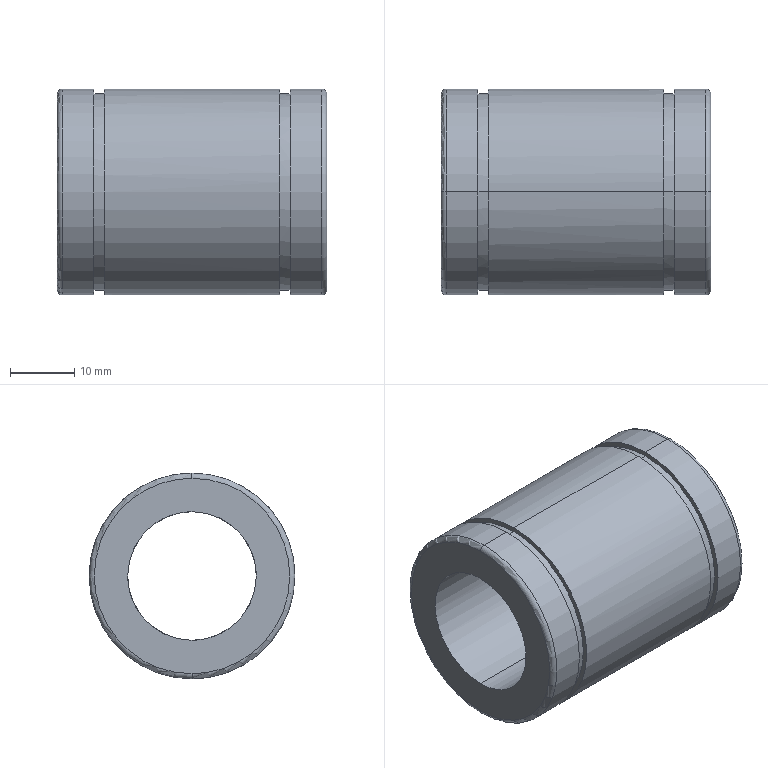Part | STEP file | _LMU-N20 | 1 solid | 22 faces | box 42 x 32 x 32 mm | volume 20321 mm3 | cylinder 12 | plane 6 | torus 4 | commonest cylinder face diameters 32 x6 30.5 x4 20 x2
STEP:
#1=CARTESIAN_POINT('',(0.,0.,-15.2));
#2=VERTEX_POINT('',#1);
#3=CARTESIAN_POINT('',(0.,15.2,0.));
#4=VERTEX_POINT('',#3);
#5=CARTESIAN_POINT('',(0.,0.,-15.2));
#6=CARTESIAN_POINT('',(0.,1.337,-15.2));
#7=CARTESIAN_POINT('',(0.,2.673,-15.053));
#8=CARTESIAN_POINT('',(0.,3.989,-14.759));
#9=CARTESIAN_POINT('',(0.,6.715,-13.825));
#10=CARTESIAN_POINT('',(0.,9.154,-12.28));
#11=CARTESIAN_POINT('',(0.,10.344,-11.295));
#12=CARTESIAN_POINT('',(0.,12.451,-9.049));
#13=CARTESIAN_POINT('',(0.,13.937,-6.351));
#14=CARTESIAN_POINT('',(0.,14.506,-4.915));
#15=CARTESIAN_POINT('',(0.,14.984,-3.05));
#16=CARTESIAN_POINT('',(0.,15.164,-1.147));
#17=CARTESIAN_POINT('',(0.,15.188,-0.7649));
#18=CARTESIAN_POINT('',(0.,15.2,-0.3824));
#19=CARTESIAN_POINT('',(0.,15.2,0.));
#20=B_SPLINE_CURVE_WITH_KNOTS('',5,(#5,#6,#7,#8,#9,#10,#11,#12,#13,#14,#15,#16,#17,#18,#19),.UNSPECIFIED.,.F.,.U.,(6,3,3,3,6),(33.766,43.217,54.022,64.826,67.53),.UNSPECIFIED.);
#21=EDGE_CURVE('',#2,#4,#20,.T.);
#22=ORIENTED_EDGE('',*,*,#21,.F.);
#23=CARTESIAN_POINT('',(0.,-15.2,0.));
#24=VERTEX_POINT('',#23);
#25=CARTESIAN_POINT('',(0.,-15.2,0.));
#26=CARTESIAN_POINT('',(0.,-15.2,-1.528));
#27=CARTESIAN_POINT('',(0.,-15.008,-3.056));
#28=CARTESIAN_POINT('',(0.,-14.624,-4.552));
#29=CARTESIAN_POINT('',(0.,-13.488,-7.415));
#30=CARTESIAN_POINT('',(0.,-11.68,-9.908));
#31=CARTESIAN_POINT('',(0.,-10.623,-11.034));
#32=CARTESIAN_POINT('',(0.,-8.248,-12.995));
#33=CARTESIAN_POINT('',(0.,-5.462,-14.309));
#34=CARTESIAN_POINT('',(0.,-3.994,-14.786));
#35=CARTESIAN_POINT('',(0.,-2.291,-15.11));
#36=CARTESIAN_POINT('',(0.,-0.5738,-15.191));
#37=CARTESIAN_POINT('',(0.,-0.3826,-15.197));
#38=CARTESIAN_POINT('',(0.,-0.1913,-15.2));
#39=CARTESIAN_POINT('',(0.,0.,-15.2));
#40=B_SPLINE_CURVE_WITH_KNOTS('',5,(#25,#26,#27,#28,#29,#30,#31,#32,#33,#34,#35,#36,#37,#38,#39),.UNSPECIFIED.,.F.,.U.,(6,3,3,3,6),(0.,10.804,21.609,32.413,33.766),.UNSPECIFIED.);
#41=EDGE_CURVE('',#24,#2,#40,.T.);
#42=ORIENTED_EDGE('',*,*,#41,.F.);
#43=CARTESIAN_POINT('',(0.,0.,15.2));
#44=VERTEX_POINT('',#43);
#45=CARTESIAN_POINT('',(0.,0.,15.2));
#46=CARTESIAN_POINT('',(0.,-1.337,15.2));
#47=CARTESIAN_POINT('',(0.,-2.673,15.053));
#48=CARTESIAN_POINT('',(0.,-3.989,14.759));
#49=CARTESIAN_POINT('',(0.,-6.715,13.825));
#50=CARTESIAN_POINT('',(0.,-9.154,12.28));
#51=CARTESIAN_POINT('',(0.,-10.344,11.295));
#52=CARTESIAN_POINT('',(0.,-12.451,9.049));
#53=CARTESIAN_POINT('',(0.,-13.937,6.351));
#54=CARTESIAN_POINT('',(0.,-14.506,4.915));
#55=CARTESIAN_POINT('',(0.,-14.984,3.05));
#56=CARTESIAN_POINT('',(0.,-15.164,1.147));
#57=CARTESIAN_POINT('',(0.,-15.188,0.7649));
#58=CARTESIAN_POINT('',(0.,-15.2,0.3824));
#59=CARTESIAN_POINT('',(0.,-15.2,0.));
#60=B_SPLINE_CURVE_WITH_KNOTS('',5,(#45,#46,#47,#48,#49,#50,#51,#52,#53,#54,#55,#56,#57,#58,#59),.UNSPECIFIED.,.F.,.U.,(6,3,3,3,6),(33.766,43.217,54.022,64.826,67.53),.UNSPECIFIED.);
#61=EDGE_CURVE('',#44,#24,#60,.T.);
#62=ORIENTED_EDGE('',*,*,#61,.F.);
#63=CARTESIAN_POINT('',(0.,15.2,0.));
#64=CARTESIAN_POINT('',(0.,15.2,1.528));
#65=CARTESIAN_POINT('',(0.,15.008,3.056));
#66=CARTESIAN_POINT('',(0.,14.624,4.552));
#67=CARTESIAN_POINT('',(0.,13.488,7.415));
#68=CARTESIAN_POINT('',(0.,11.68,9.908));
#69=CARTESIAN_POINT('',(0.,10.623,11.034));
#70=CARTESIAN_POINT('',(0.,8.248,12.995));
#71=CARTESIAN_POINT('',(0.,5.462,14.309));
#72=CARTESIAN_POINT('',(0.,3.994,14.786));
#73=CARTESIAN_POINT('',(0.,2.291,15.11));
#74=CARTESIAN_POINT('',(0.,0.5738,15.191));
#75=CARTESIAN_POINT('',(0.,0.3826,15.197));
#76=CARTESIAN_POINT('',(0.,0.1913,15.2));
#77=CARTESIAN_POINT('',(0.,0.,15.2));
#78=B_SPLINE_CURVE_WITH_KNOTS('',5,(#63,#64,#65,#66,#67,#68,#69,#70,#71,#72,#73,#74,#75,#76,#77),.UNSPECIFIED.,.F.,.U.,(6,3,3,3,6),(0.,10.804,21.609,32.413,33.766),.UNSPECIFIED.);
#79=EDGE_CURVE('',#4,#44,#78,.T.);
#80=ORIENTED_EDGE('',*,*,#79,.F.);
#81=EDGE_LOOP('',(#22,#42,#62,#80));
#82=FACE_OUTER_BOUND('',#81,.T.);
#83=CARTESIAN_POINT('',(0.,10.,0.));
#84=VERTEX_POINT('',#83);
#85=CARTESIAN_POINT('',(0.,0.,10.));
#86=VERTEX_POINT('',#85);
#87=CARTESIAN_POINT('',(0.,10.,0.));
#88=CARTESIAN_POINT('',(0.,10.,0.9295));
#89=CARTESIAN_POINT('',(0.,9.892,1.859));
#90=CARTESIAN_POINT('',(0.,9.676,2.772));
#91=CARTESIAN_POINT('',(0.,9.036,4.53));
#92=CARTESIAN_POINT('',(0.,8.01,6.095));
#93=CARTESIAN_POINT('',(0.,7.407,6.815));
#94=CARTESIAN_POINT('',(0.,6.047,8.1));
#95=CARTESIAN_POINT('',(0.,4.428,9.039));
#96=CARTESIAN_POINT('',(0.,3.567,9.412));
#97=CARTESIAN_POINT('',(0.,2.331,9.784));
#98=CARTESIAN_POINT('',(0.,1.058,9.953));
#99=CARTESIAN_POINT('',(0.,0.7061,9.984));
#100=CARTESIAN_POINT('',(0.,0.353,10.));
#101=CARTESIAN_POINT('',(0.,0.,10.));
#102=B_SPLINE_CURVE_WITH_KNOTS('',5,(#87,#88,#89,#90,#91,#92,#93,#94,#95,#96,#97,#98,#99,#100,#101),.UNSPECIFIED.,.F.,.U.,(6,3,3,3,6),(0.,6.573,13.145,19.718,22.214),.UNSPECIFIED.);
#103=EDGE_CURVE('',#84,#86,#102,.T.);
#104=ORIENTED_EDGE('',*,*,#103,.T.);
#105=CARTESIAN_POINT('',(0.,-10.,0.));
#106=VERTEX_POINT('',#105);
#107=CARTESIAN_POINT('',(0.,0.,10.));
#108=CARTESIAN_POINT('',(0.,-0.5765,10.));
#109=CARTESIAN_POINT('',(0.,-1.153,9.958));
#110=CARTESIAN_POINT('',(0.,-1.725,9.875));
#111=CARTESIAN_POINT('',(0.,-3.2,9.551));
#112=CARTESIAN_POINT('',(0.,-4.594,8.955));
#113=CARTESIAN_POINT('',(0.,-5.408,8.489));
#114=CARTESIAN_POINT('',(0.,-6.912,7.375));
#115=CARTESIAN_POINT('',(0.,-8.121,5.946));
#116=CARTESIAN_POINT('',(0.,-8.639,5.165));
#117=CARTESIAN_POINT('',(0.,-9.383,3.696));
#118=CARTESIAN_POINT('',(0.,-9.813,2.111));
#119=CARTESIAN_POINT('',(0.,-9.938,1.412));
#120=CARTESIAN_POINT('',(0.,-10.,0.7061));
#121=CARTESIAN_POINT('',(0.,-10.,0.));
#122=B_SPLINE_CURVE_WITH_KNOTS('',5,(#107,#108,#109,#110,#111,#112,#113,#114,#115,#116,#117,#118,#119,#120,#121),.UNSPECIFIED.,.F.,.U.,(6,3,3,3,6),(22.214,26.29,32.863,39.436,44.428),.UNSPECIFIED.);
#123=EDGE_CURVE('',#86,#106,#122,.T.);
#124=ORIENTED_EDGE('',*,*,#123,.T.);
#125=CARTESIAN_POINT('',(0.,0.,-10.));
#126=VERTEX_POINT('',#125);
#127=CARTESIAN_POINT('',(0.,-10.,0.));
#128=CARTESIAN_POINT('',(0.,-10.,-0.9295));
#129=CARTESIAN_POINT('',(0.,-9.892,-1.859));
#130=CARTESIAN_POINT('',(0.,-9.676,-2.772));
#131=CARTESIAN_POINT('',(0.,-9.036,-4.53));
#132=CARTESIAN_POINT('',(0.,-8.01,-6.095));
#133=CARTESIAN_POINT('',(0.,-7.407,-6.815));
#134=CARTESIAN_POINT('',(0.,-6.047,-8.1));
#135=CARTESIAN_POINT('',(0.,-4.428,-9.039));
#136=CARTESIAN_POINT('',(0.,-3.567,-9.412));
#137=CARTESIAN_POINT('',(0.,-2.331,-9.784));
#138=CARTESIAN_POINT('',(0.,-1.058,-9.953));
#139=CARTESIAN_POINT('',(0.,-0.7061,-9.984));
#140=CARTESIAN_POINT('',(0.,-0.353,-10.));
#141=CARTESIAN_POINT('',(0.,0.,-10.));
#142=B_SPLINE_CURVE_WITH_KNOTS('',5,(#127,#128,#129,#130,#131,#132,#133,#134,#135,#136,#137,#138,#139,#140,#141),.UNSPECIFIED.,.F.,.U.,(6,3,3,3,6),(0.,6.573,13.145,19.718,22.214),.UNSPECIFIED.);
#143=EDGE_CURVE('',#106,#126,#142,.T.);
#144=ORIENTED_EDGE('',*,*,#143,.T.);
#145=CARTESIAN_POINT('',(0.,0.,-10.));
#146=CARTESIAN_POINT('',(0.,0.5765,-10.));
#147=CARTESIAN_POINT('',(0.,1.153,-9.958));
#148=CARTESIAN_POINT('',(0.,1.725,-9.875));
#149=CARTESIAN_POINT('',(0.,3.2,-9.551));
#150=CARTESIAN_POINT('',(0.,4.594,-8.955));
#151=CARTESIAN_POINT('',(0.,5.408,-8.489));
#152=CARTESIAN_POINT('',(0.,6.912,-7.375));
#153=CARTESIAN_POINT('',(0.,8.121,-5.946));
#154=CARTESIAN_POINT('',(0.,8.639,-5.165));
#155=CARTESIAN_POINT('',(0.,9.383,-3.696));
#156=CARTESIAN_POINT('',(0.,9.813,-2.111));
#157=CARTESIAN_POINT('',(0.,9.938,-1.412));
#158=CARTESIAN_POINT('',(0.,10.,-0.7061));
#159=CARTESIAN_POINT('',(0.,10.,0.));
#160=B_SPLINE_CURVE_WITH_KNOTS('',5,(#145,#146,#147,#148,#149,#150,#151,#152,#153,#154,#155,#156,#157,#158,#159),.UNSPECIFIED.,.F.,.U.,(6,3,3,3,6),(22.214,26.29,32.863,39.436,44.428),.UNSPECIFIED.);
#161=EDGE_CURVE('',#126,#84,#160,.T.);
#162=ORIENTED_EDGE('',*,*,#161,.T.);
#163=EDGE_LOOP('',(#104,#124,#144,#162));
#164=FACE_BOUND('',#163,.T.);
#165=CARTESIAN_POINT('',(0.,15.2,0.));
#166=DIRECTION('',(-1.,0.,0.));
#167=DIRECTION('',(0.,0.,1.));
#168=AXIS2_PLACEMENT_3D('',#165,#166,#167);
#169=PLANE('',#168);
#170=ADVANCED_FACE('',(#82,#164),#169,.T.);
#171=CARTESIAN_POINT('',(0.8,0.,16.));
#172=VERTEX_POINT('',#171);
#173=CARTESIAN_POINT('',(0.8,0.,15.2));
#174=DIRECTION('',(0.,1.,0.));
#175=AXIS2_PLACEMENT_3D('',#173,#174,$);
#176=CIRCLE('',#175,0.8);
#177=EDGE_CURVE('',#44,#172,#176,.T.);
#178=ORIENTED_EDGE('',*,*,#177,.T.);
#179=CARTESIAN_POINT('',(0.8,16.,0.));
#180=VERTEX_POINT('',#179);
#181=CARTESIAN_POINT('',(0.8,0.,0.));
#182=DIRECTION('',(1.,0.,0.));
#183=AXIS2_PLACEMENT_3D('',#181,#182,$);
#184=CIRCLE('',#183,16.);
#185=EDGE_CURVE('',#180,#172,#184,.T.);
#186=ORIENTED_EDGE('',*,*,#185,.F.);
#187=CARTESIAN_POINT('',(0.8,0.,-16.));
#188=VERTEX_POINT('',#187);
#189=CARTESIAN_POINT('',(0.8,0.,0.));
#190=DIRECTION('',(1.,0.,0.));
#191=AXIS2_PLACEMENT_3D('',#189,#190,$);
#192=CIRCLE('',#191,16.);
#193=EDGE_CURVE('',#188,#180,#192,.T.);
#194=ORIENTED_EDGE('',*,*,#193,.F.);
#195=CARTESIAN_POINT('',(0.8,0.,-15.2));
#196=DIRECTION('',(0.,-1.,0.));
#197=AXIS2_PLACEMENT_3D('',#195,#196,$);
#198=CIRCLE('',#197,0.8);
#199=EDGE_CURVE('',#188,#2,#198,.F.);
#200=ORIENTED_EDGE('',*,*,#199,.T.);
#201=ORIENTED_EDGE('',*,*,#21,.T.);
#202=ORIENTED_EDGE('',*,*,#79,.T.);
#203=EDGE_LOOP('',(#178,#186,#194,#200,#201,#202));
#204=FACE_OUTER_BOUND('',#203,.T.);
#205=CARTESIAN_POINT('',(0.8,0.,0.));
#206=DIRECTION('',(1.,0.,0.));
#207=DIRECTION('',(0.,0.,-1.));
#208=AXIS2_PLACEMENT_3D('',#205,#206,#207);
#209=TOROIDAL_SURFACE('',#208,15.2,0.8);
#210=ADVANCED_FACE('',(#204),#209,.T.);
#211=ORIENTED_EDGE('',*,*,#199,.F.);
#212=CARTESIAN_POINT('',(0.8,-16.,0.));
#213=VERTEX_POINT('',#212);
#214=CARTESIAN_POINT('',(0.8,0.,0.));
#215=DIRECTION('',(1.,0.,0.));
#216=AXIS2_PLACEMENT_3D('',#214,#215,$);
#217=CIRCLE('',#216,16.);
#218=EDGE_CURVE('',#213,#188,#217,.T.);
#219=ORIENTED_EDGE('',*,*,#218,.F.);
#220=CARTESIAN_POINT('',(0.8,0.,0.));
#221=DIRECTION('',(1.,0.,0.));
#222=AXIS2_PLACEMENT_3D('',#220,#221,$);
#223=CIRCLE('',#222,16.);
#224=EDGE_CURVE('',#172,#213,#223,.T.);
#225=ORIENTED_EDGE('',*,*,#224,.F.);
#226=ORIENTED_EDGE('',*,*,#177,.F.);
#227=ORIENTED_EDGE('',*,*,#61,.T.);
#228=ORIENTED_EDGE('',*,*,#41,.T.);
#229=EDGE_LOOP('',(#211,#219,#225,#226,#227,#228));
#230=FACE_OUTER_BOUND('',#229,.T.);
#231=CARTESIAN_POINT('',(0.8,0.,0.));
#232=DIRECTION('',(1.,0.,0.));
#233=DIRECTION('',(0.,0.,1.));
#234=AXIS2_PLACEMENT_3D('',#231,#232,#233);
#235=TOROIDAL_SURFACE('',#234,15.2,0.8);
#236=ADVANCED_FACE('',(#230),#235,.T.);
#237=CARTESIAN_POINT('',(42.,0.,-10.));
#238=VERTEX_POINT('',#237);
#239=CARTESIAN_POINT('',(42.,10.,0.));
#240=VERTEX_POINT('',#239);
#241=CARTESIAN_POINT('',(42.,0.,0.));
#242=DIRECTION('',(-1.,0.,0.));
#243=AXIS2_PLACEMENT_3D('',#241,#242,$);
#244=CIRCLE('',#243,10.);
#245=EDGE_CURVE('',#238,#240,#244,.F.);
#246=ORIENTED_EDGE('',*,*,#245,.T.);
#247=CARTESIAN_POINT('',(42.,0.,10.));
#248=VERTEX_POINT('',#247);
#249=CARTESIAN_POINT('',(42.,0.,0.));
#250=DIRECTION('',(-1.,0.,0.));
#251=AXIS2_PLACEMENT_3D('',#249,#250,$);
#252=CIRCLE('',#251,10.);
#253=EDGE_CURVE('',#240,#248,#252,.F.);
#254=ORIENTED_EDGE('',*,*,#253,.T.);
#255=CARTESIAN_POINT('',(42.,0.,10.));
#256=DIRECTION('',(-1.,0.,0.));
#257=VECTOR('',#256,1.);
#258=LINE('',#255,#257);
#259=EDGE_CURVE('',#248,#86,#258,.T.);
#260=ORIENTED_EDGE('',*,*,#259,.T.);
#261=ORIENTED_EDGE('',*,*,#103,.F.);
#262=ORIENTED_EDGE('',*,*,#161,.F.);
#263=CARTESIAN_POINT('',(42.,0.,-10.));
#264=DIRECTION('',(-1.,0.,0.));
#265=VECTOR('',#264,1.);
#266=LINE('',#263,#265);
#267=EDGE_CURVE('',#126,#238,#266,.F.);
#268=ORIENTED_EDGE('',*,*,#267,.T.);
#269=EDGE_LOOP('',(#246,#254,#260,#261,#262,#268));
#270=FACE_OUTER_BOUND('',#269,.T.);
#271=CARTESIAN_POINT('',(42.,0.,0.));
#272=DIRECTION('',(-1.,0.,0.));
#273=DIRECTION('',(0.,0.,1.));
#274=AXIS2_PLACEMENT_3D('',#271,#272,#273);
#275=CYLINDRICAL_SURFACE('',#274,10.);
#276=ADVANCED_FACE('',(#270),#275,.F.);
#277=CARTESIAN_POINT('',(42.,-10.,0.));
#278=VERTEX_POINT('',#277);
#279=CARTESIAN_POINT('',(42.,0.,0.));
#280=DIRECTION('',(-1.,0.,0.));
#281=AXIS2_PLACEMENT_3D('',#279,#280,$);
#282=CIRCLE('',#281,10.);
#283=EDGE_CURVE('',#248,#278,#282,.F.);
#284=ORIENTED_EDGE('',*,*,#283,.T.);
#285=CARTESIAN_POINT('',(42.,0.,0.));
#286=DIRECTION('',(-1.,0.,0.));
#287=AXIS2_PLACEMENT_3D('',#285,#286,$);
#288=CIRCLE('',#287,10.);
#289=EDGE_CURVE('',#278,#238,#288,.F.);
#290=ORIENTED_EDGE('',*,*,#289,.T.);
#291=ORIENTED_EDGE('',*,*,#267,.F.);
#292=ORIENTED_EDGE('',*,*,#143,.F.);
#293=ORIENTED_EDGE('',*,*,#123,.F.);
#294=ORIENTED_EDGE('',*,*,#259,.F.);
#295=EDGE_LOOP('',(#284,#290,#291,#292,#293,#294));
#296=FACE_OUTER_BOUND('',#295,.T.);
#297=CARTESIAN_POINT('',(42.,0.,0.));
#298=DIRECTION('',(-1.,0.,0.));
#299=DIRECTION('',(0.,0.,-1.));
#300=AXIS2_PLACEMENT_3D('',#297,#298,#299);
#301=CYLINDRICAL_SURFACE('',#300,10.);
#302=ADVANCED_FACE('',(#296),#301,.F.);
#303=CARTESIAN_POINT('',(5.75,0.,16.));
#304=VERTEX_POINT('',#303);
#305=CARTESIAN_POINT('',(42.,0.,16.));
#306=DIRECTION('',(-1.,0.,0.));
#307=VECTOR('',#306,1.);
#308=LINE('',#305,#307);
#309=EDGE_CURVE('',#304,#172,#308,.T.);
#310=ORIENTED_EDGE('',*,*,#309,.F.);
#311=CARTESIAN_POINT('',(5.75,16.,0.));
#312=VERTEX_POINT('',#311);
#313=CARTESIAN_POINT('',(5.75,0.,0.));
#314=DIRECTION('',(-1.,0.,0.));
#315=AXIS2_PLACEMENT_3D('',#313,#314,$);
#316=CIRCLE('',#315,16.);
#317=EDGE_CURVE('',#312,#304,#316,.F.);
#318=ORIENTED_EDGE('',*,*,#317,.F.);
#319=CARTESIAN_POINT('',(5.75,0.,-16.));
#320=VERTEX_POINT('',#319);
#321=CARTESIAN_POINT('',(5.75,0.,0.));
#322=DIRECTION('',(-1.,0.,0.));
#323=AXIS2_PLACEMENT_3D('',#321,#322,$);
#324=CIRCLE('',#323,16.);
#325=EDGE_CURVE('',#320,#312,#324,.F.);
#326=ORIENTED_EDGE('',*,*,#325,.F.);
#327=CARTESIAN_POINT('',(42.,0.,-16.));
#328=DIRECTION('',(-1.,0.,0.));
#329=VECTOR('',#328,1.);
#330=LINE('',#327,#329);
#331=EDGE_CURVE('',#188,#320,#330,.F.);
#332=ORIENTED_EDGE('',*,*,#331,.F.);
#333=ORIENTED_EDGE('',*,*,#193,.T.);
#334=ORIENTED_EDGE('',*,*,#185,.T.);
#335=EDGE_LOOP('',(#310,#318,#326,#332,#333,#334));
#336=FACE_OUTER_BOUND('',#335,.T.);
#337=CARTESIAN_POINT('',(42.,0.,0.));
#338=DIRECTION('',(-1.,0.,0.));
#339=DIRECTION('',(0.,0.,1.));
#340=AXIS2_PLACEMENT_3D('',#337,#338,#339);
#341=CYLINDRICAL_SURFACE('',#340,16.);
#342=ADVANCED_FACE('',(#336),#341,.T.);
#343=ORIENTED_EDGE('',*,*,#331,.T.);
#344=CARTESIAN_POINT('',(5.75,-16.,0.));
#345=VERTEX_POINT('',#344);
#346=CARTESIAN_POINT('',(5.75,0.,0.));
#347=DIRECTION('',(-1.,0.,0.));
#348=AXIS2_PLACEMENT_3D('',#346,#347,$);
#349=CIRCLE('',#348,16.);
#350=EDGE_CURVE('',#345,#320,#349,.F.);
#351=ORIENTED_EDGE('',*,*,#350,.F.);
#352=CARTESIAN_POINT('',(5.75,0.,0.));
#353=DIRECTION('',(-1.,0.,0.));
#354=AXIS2_PLACEMENT_3D('',#352,#353,$);
#355=CIRCLE('',#354,16.);
#356=EDGE_CURVE('',#304,#345,#355,.F.);
#357=ORIENTED_EDGE('',*,*,#356,.F.);
#358=ORIENTED_EDGE('',*,*,#309,.T.);
#359=ORIENTED_EDGE('',*,*,#224,.T.);
#360=ORIENTED_EDGE('',*,*,#218,.T.);
#361=EDGE_LOOP('',(#343,#351,#357,#358,#359,#360));
#362=FACE_OUTER_BOUND('',#361,.T.);
#363=CARTESIAN_POINT('',(42.,0.,0.));
#364=DIRECTION('',(-1.,0.,0.));
#365=DIRECTION('',(0.,0.,-1.));
#366=AXIS2_PLACEMENT_3D('',#363,#364,#365);
#367=CYLINDRICAL_SURFACE('',#366,16.);
#368=ADVANCED_FACE('',(#362),#367,.T.);
#369=CARTESIAN_POINT('',(42.,15.2,0.));
#370=VERTEX_POINT('',#369);
#371=CARTESIAN_POINT('',(42.,0.,15.2));
#372=VERTEX_POINT('',#371);
#373=CARTESIAN_POINT('',(42.,0.,0.));
#374=DIRECTION('',(1.,0.,0.));
#375=AXIS2_PLACEMENT_3D('',#373,#374,$);
#376=CIRCLE('',#375,15.2);
#377=EDGE_CURVE('',#370,#372,#376,.T.);
#378=ORIENTED_EDGE('',*,*,#377,.T.);
#379=CARTESIAN_POINT('',(42.,-15.2,0.));
#380=VERTEX_POINT('',#379);
#381=CARTESIAN_POINT('',(42.,0.,0.));
#382=DIRECTION('',(1.,0.,0.));
#383=AXIS2_PLACEMENT_3D('',#381,#382,$);
#384=CIRCLE('',#383,15.2);
#385=EDGE_CURVE('',#372,#380,#384,.T.);
#386=ORIENTED_EDGE('',*,*,#385,.T.);
#387=CARTESIAN_POINT('',(42.,0.,-15.2));
#388=VERTEX_POINT('',#387);
#389=CARTESIAN_POINT('',(42.,0.,0.));
#390=DIRECTION('',(1.,0.,0.));
#391=AXIS2_PLACEMENT_3D('',#389,#390,$);
#392=CIRCLE('',#391,15.2);
#393=EDGE_CURVE('',#380,#388,#392,.T.);
#394=ORIENTED_EDGE('',*,*,#393,.T.);
#395=CARTESIAN_POINT('',(42.,0.,0.));
#396=DIRECTION('',(1.,0.,0.));
#397=AXIS2_PLACEMENT_3D('',#395,#396,$);
#398=CIRCLE('',#397,15.2);
#399=EDGE_CURVE('',#388,#370,#398,.T.);
#400=ORIENTED_EDGE('',*,*,#399,.T.);
#401=EDGE_LOOP('',(#378,#386,#394,#400));
#402=FACE_OUTER_BOUND('',#401,.T.);
#403=ORIENTED_EDGE('',*,*,#245,.F.);
#404=ORIENTED_EDGE('',*,*,#289,.F.);
#405=ORIENTED_EDGE('',*,*,#283,.F.);
#406=ORIENTED_EDGE('',*,*,#253,.F.);
#407=EDGE_LOOP('',(#403,#404,#405,#406));
#408=FACE_BOUND('',#407,.T.);
#409=CARTESIAN_POINT('',(42.,10.,0.));
#410=DIRECTION('',(1.,0.,0.));
#411=DIRECTION('',(0.,0.,-1.));
#412=AXIS2_PLACEMENT_3D('',#409,#410,#411);
#413=PLANE('',#412);
#414=ADVANCED_FACE('',(#402,#408),#413,.T.);
#415=ORIENTED_EDGE('',*,*,#317,.T.);
#416=ORIENTED_EDGE('',*,*,#356,.T.);
#417=ORIENTED_EDGE('',*,*,#350,.T.);
#418=ORIENTED_EDGE('',*,*,#325,.T.);
#419=EDGE_LOOP('',(#415,#416,#417,#418));
#420=FACE_OUTER_BOUND('',#419,.T.);
#421=CARTESIAN_POINT('',(5.75,0.,-15.25));
#422=VERTEX_POINT('',#421);
#423=CARTESIAN_POINT('',(5.75,15.25,0.));
#424=VERTEX_POINT('',#423);
#425=CARTESIAN_POINT('',(5.75,0.,0.));
#426=DIRECTION('',(1.,0.,0.));
#427=AXIS2_PLACEMENT_3D('',#425,#426,$);
#428=CIRCLE('',#427,15.25);
#429=EDGE_CURVE('',#422,#424,#428,.T.);
#430=ORIENTED_EDGE('',*,*,#429,.F.);
#431=CARTESIAN_POINT('',(5.75,-15.25,0.));
#432=VERTEX_POINT('',#431);
#433=CARTESIAN_POINT('',(5.75,0.,0.));
#434=DIRECTION('',(1.,0.,0.));
#435=AXIS2_PLACEMENT_3D('',#433,#434,$);
#436=CIRCLE('',#435,15.25);
#437=EDGE_CURVE('',#432,#422,#436,.T.);
#438=ORIENTED_EDGE('',*,*,#437,.F.);
#439=CARTESIAN_POINT('',(5.75,0.,15.25));
#440=VERTEX_POINT('',#439);
#441=CARTESIAN_POINT('',(5.75,0.,0.));
#442=DIRECTION('',(1.,0.,0.));
#443=AXIS2_PLACEMENT_3D('',#441,#442,$);
#444=CIRCLE('',#443,15.25);
#445=EDGE_CURVE('',#440,#432,#444,.T.);
#446=ORIENTED_EDGE('',*,*,#445,.F.);
#447=CARTESIAN_POINT('',(5.75,0.,0.));
#448=DIRECTION('',(1.,0.,0.));
#449=AXIS2_PLACEMENT_3D('',#447,#448,$);
#450=CIRCLE('',#449,15.25);
#451=EDGE_CURVE('',#424,#440,#450,.T.);
#452=ORIENTED_EDGE('',*,*,#451,.F.);
#453=EDGE_LOOP('',(#430,#438,#446,#452));
#454=FACE_BOUND('',#453,.T.);
#455=CARTESIAN_POINT('',(5.75,15.25,0.));
#456=DIRECTION('',(1.,0.,0.));
#457=DIRECTION('',(0.,0.,-1.));
#458=AXIS2_PLACEMENT_3D('',#455,#456,#457);
#459=PLANE('',#458);
#460=ADVANCED_FACE('',(#420,#454),#459,.T.);
#461=CARTESIAN_POINT('',(41.2,0.,16.));
#462=VERTEX_POINT('',#461);
#463=CARTESIAN_POINT('',(41.2,0.,15.2));
#464=DIRECTION('',(0.,1.,0.));
#465=AXIS2_PLACEMENT_3D('',#463,#464,$);
#466=CIRCLE('',#465,0.8);
#467=EDGE_CURVE('',#462,#372,#466,.T.);
#468=ORIENTED_EDGE('',*,*,#467,.T.);
#469=ORIENTED_EDGE('',*,*,#377,.F.);
#470=ORIENTED_EDGE('',*,*,#399,.F.);
#471=CARTESIAN_POINT('',(41.2,0.,-16.));
#472=VERTEX_POINT('',#471);
#473=CARTESIAN_POINT('',(41.2,0.,-15.2));
#474=DIRECTION('',(0.,-1.,0.));
#475=AXIS2_PLACEMENT_3D('',#473,#474,$);
#476=CIRCLE('',#475,0.8);
#477=EDGE_CURVE('',#388,#472,#476,.F.);
#478=ORIENTED_EDGE('',*,*,#477,.T.);
#479=CARTESIAN_POINT('',(41.2,16.,0.));
#480=VERTEX_POINT('',#479);
#481=CARTESIAN_POINT('',(41.2,0.,0.));
#482=DIRECTION('',(1.,0.,0.));
#483=AXIS2_PLACEMENT_3D('',#481,#482,$);
#484=CIRCLE('',#483,16.);
#485=EDGE_CURVE('',#472,#480,#484,.T.);
#486=ORIENTED_EDGE('',*,*,#485,.T.);
#487=CARTESIAN_POINT('',(41.2,0.,0.));
#488=DIRECTION('',(1.,0.,0.));
#489=AXIS2_PLACEMENT_3D('',#487,#488,$);
#490=CIRCLE('',#489,16.);
#491=EDGE_CURVE('',#480,#462,#490,.T.);
#492=ORIENTED_EDGE('',*,*,#491,.T.);
#493=EDGE_LOOP('',(#468,#469,#470,#478,#486,#492));
#494=FACE_OUTER_BOUND('',#493,.T.);
#495=CARTESIAN_POINT('',(41.2,0.,0.));
#496=DIRECTION('',(1.,0.,0.));
#497=DIRECTION('',(0.,0.,-1.));
#498=AXIS2_PLACEMENT_3D('',#495,#496,#497);
#499=TOROIDAL_SURFACE('',#498,15.2,0.8);
#500=ADVANCED_FACE('',(#494),#499,.T.);
#501=ORIENTED_EDGE('',*,*,#477,.F.);
#502=ORIENTED_EDGE('',*,*,#393,.F.);
#503=ORIENTED_EDGE('',*,*,#385,.F.);
#504=ORIENTED_EDGE('',*,*,#467,.F.);
#505=CARTESIAN_POINT('',(41.2,-16.,0.));
#506=VERTEX_POINT('',#505);
#507=CARTESIAN_POINT('',(41.2,0.,0.));
#508=DIRECTION('',(1.,0.,0.));
#509=AXIS2_PLACEMENT_3D('',#507,#508,$);
#510=CIRCLE('',#509,16.);
#511=EDGE_CURVE('',#462,#506,#510,.T.);
#512=ORIENTED_EDGE('',*,*,#511,.T.);
#513=CARTESIAN_POINT('',(41.2,0.,0.));
#514=DIRECTION('',(1.,0.,0.));
#515=AXIS2_PLACEMENT_3D('',#513,#514,$);
#516=CIRCLE('',#515,16.);
#517=EDGE_CURVE('',#506,#472,#516,.T.);
#518=ORIENTED_EDGE('',*,*,#517,.T.);
#519=EDGE_LOOP('',(#501,#502,#503,#504,#512,#518));
#520=FACE_OUTER_BOUND('',#519,.T.);
#521=CARTESIAN_POINT('',(41.2,0.,0.));
#522=DIRECTION('',(1.,0.,0.));
#523=DIRECTION('',(0.,0.,1.));
#524=AXIS2_PLACEMENT_3D('',#521,#522,#523);
#525=TOROIDAL_SURFACE('',#524,15.2,0.8);
#526=ADVANCED_FACE('',(#520),#525,.T.);
#527=CARTESIAN_POINT('',(7.35,0.,15.25));
#528=VERTEX_POINT('',#527);
#529=CARTESIAN_POINT('',(42.,0.,15.25));
#530=DIRECTION('',(-1.,0.,0.));
#531=VECTOR('',#530,1.);
#532=LINE('',#529,#531);
#533=EDGE_CURVE('',#528,#440,#532,.T.);
#534=ORIENTED_EDGE('',*,*,#533,.F.);
#535=CARTESIAN_POINT('',(7.35,15.25,0.));
#536=VERTEX_POINT('',#535);
#537=CARTESIAN_POINT('',(7.35,15.25,0.));
#538=CARTESIAN_POINT('',(7.35,15.25,4.791));
#539=CARTESIAN_POINT('',(7.35,13.374,9.586));
#540=CARTESIAN_POINT('',(7.35,9.586,13.374));
#541=CARTESIAN_POINT('',(7.35,4.791,15.25));
#542=CARTESIAN_POINT('',(7.35,0.,15.25));
#543=B_SPLINE_CURVE_WITH_KNOTS('',5,(#537,#538,#539,#540,#541,#542),.UNSPECIFIED.,.F.,.U.,(6,6),(-11.977,11.977),.UNSPECIFIED.);
#544=EDGE_CURVE('',#536,#528,#543,.T.);
#545=ORIENTED_EDGE('',*,*,#544,.F.);
#546=CARTESIAN_POINT('',(7.35,0.,-15.25));
#547=VERTEX_POINT('',#546);
#548=CARTESIAN_POINT('',(7.35,0.,0.));
#549=DIRECTION('',(-1.,0.,0.));
#550=AXIS2_PLACEMENT_3D('',#548,#549,$);
#551=CIRCLE('',#550,15.25);
#552=EDGE_CURVE('',#547,#536,#551,.F.);
#553=ORIENTED_EDGE('',*,*,#552,.F.);
#554=CARTESIAN_POINT('',(42.,0.,-15.25));
#555=DIRECTION('',(-1.,0.,0.));
#556=VECTOR('',#555,1.);
#557=LINE('',#554,#556);
#558=EDGE_CURVE('',#422,#547,#557,.F.);
#559=ORIENTED_EDGE('',*,*,#558,.F.);
#560=ORIENTED_EDGE('',*,*,#429,.T.);
#561=ORIENTED_EDGE('',*,*,#451,.T.);
#562=EDGE_LOOP('',(#534,#545,#553,#559,#560,#561));
#563=FACE_OUTER_BOUND('',#562,.T.);
#564=CARTESIAN_POINT('',(42.,0.,0.));
#565=DIRECTION('',(-1.,0.,0.));
#566=DIRECTION('',(0.,0.,1.));
#567=AXIS2_PLACEMENT_3D('',#564,#565,#566);
#568=CYLINDRICAL_SURFACE('',#567,15.25);
#569=ADVANCED_FACE('',(#563),#568,.T.);
#570=ORIENTED_EDGE('',*,*,#558,.T.);
#571=CARTESIAN_POINT('',(7.35,-15.25,0.));
#572=VERTEX_POINT('',#571);
#573=CARTESIAN_POINT('',(7.35,0.,0.));
#574=DIRECTION('',(-1.,0.,0.));
#575=AXIS2_PLACEMENT_3D('',#573,#574,$);
#576=CIRCLE('',#575,15.25);
#577=EDGE_CURVE('',#572,#547,#576,.F.);
#578=ORIENTED_EDGE('',*,*,#577,.F.);
#579=CARTESIAN_POINT('',(7.35,0.,15.25));
#580=CARTESIAN_POINT('',(7.35,-4.791,15.25));
#581=CARTESIAN_POINT('',(7.35,-9.586,13.374));
#582=CARTESIAN_POINT('',(7.35,-13.374,9.586));
#583=CARTESIAN_POINT('',(7.35,-15.25,4.791));
#584=CARTESIAN_POINT('',(7.35,-15.25,0.));
#585=B_SPLINE_CURVE_WITH_KNOTS('',5,(#579,#580,#581,#582,#583,#584),.UNSPECIFIED.,.F.,.U.,(6,6),(-11.977,11.977),.UNSPECIFIED.);
#586=EDGE_CURVE('',#528,#572,#585,.T.);
#587=ORIENTED_EDGE('',*,*,#586,.F.);
#588=ORIENTED_EDGE('',*,*,#533,.T.);
#589=ORIENTED_EDGE('',*,*,#445,.T.);
#590=ORIENTED_EDGE('',*,*,#437,.T.);
#591=EDGE_LOOP('',(#570,#578,#587,#588,#589,#590));
#592=FACE_OUTER_BOUND('',#591,.T.);
#593=CARTESIAN_POINT('',(42.,0.,0.));
#594=DIRECTION('',(-1.,0.,0.));
#595=DIRECTION('',(0.,0.,-1.));
#596=AXIS2_PLACEMENT_3D('',#593,#594,#595);
#597=CYLINDRICAL_SURFACE('',#596,15.25);
#598=ADVANCED_FACE('',(#592),#597,.T.);
#599=CARTESIAN_POINT('',(36.25,0.,16.));
#600=VERTEX_POINT('',#599);
#601=CARTESIAN_POINT('',(42.,0.,16.));
#602=DIRECTION('',(-1.,0.,0.));
#603=VECTOR('',#602,1.);
#604=LINE('',#601,#603);
#605=EDGE_CURVE('',#462,#600,#604,.T.);
#606=ORIENTED_EDGE('',*,*,#605,.F.);
#607=ORIENTED_EDGE('',*,*,#491,.F.);
#608=ORIENTED_EDGE('',*,*,#485,.F.);
#609=CARTESIAN_POINT('',(36.25,0.,-16.));
#610=VERTEX_POINT('',#609);
#611=CARTESIAN_POINT('',(42.,0.,-16.));
#612=DIRECTION('',(-1.,0.,0.));
#613=VECTOR('',#612,1.);
#614=LINE('',#611,#613);
#615=EDGE_CURVE('',#610,#472,#614,.F.);
#616=ORIENTED_EDGE('',*,*,#615,.F.);
#617=CARTESIAN_POINT('',(36.25,16.,0.));
#618=VERTEX_POINT('',#617);
#619=CARTESIAN_POINT('',(36.25,0.,0.));
#620=DIRECTION('',(-1.,0.,0.));
#621=AXIS2_PLACEMENT_3D('',#619,#620,$);
#622=CIRCLE('',#621,16.);
#623=EDGE_CURVE('',#610,#618,#622,.F.);
#624=ORIENTED_EDGE('',*,*,#623,.T.);
#625=CARTESIAN_POINT('',(36.25,0.,0.));
#626=DIRECTION('',(-1.,0.,0.));
#627=AXIS2_PLACEMENT_3D('',#625,#626,$);
#628=CIRCLE('',#627,16.);
#629=EDGE_CURVE('',#618,#600,#628,.F.);
#630=ORIENTED_EDGE('',*,*,#629,.T.);
#631=EDGE_LOOP('',(#606,#607,#608,#616,#624,#630));
#632=FACE_OUTER_BOUND('',#631,.T.);
#633=CARTESIAN_POINT('',(42.,0.,0.));
#634=DIRECTION('',(-1.,0.,0.));
#635=DIRECTION('',(0.,0.,1.));
#636=AXIS2_PLACEMENT_3D('',#633,#634,#635);
#637=CYLINDRICAL_SURFACE('',#636,16.);
#638=ADVANCED_FACE('',(#632),#637,.T.);
#639=ORIENTED_EDGE('',*,*,#615,.T.);
#640=ORIENTED_EDGE('',*,*,#517,.F.);
#641=ORIENTED_EDGE('',*,*,#511,.F.);
#642=ORIENTED_EDGE('',*,*,#605,.T.);
#643=CARTESIAN_POINT('',(36.25,-16.,0.));
#644=VERTEX_POINT('',#643);
#645=CARTESIAN_POINT('',(36.25,0.,0.));
#646=DIRECTION('',(-1.,0.,0.));
#647=AXIS2_PLACEMENT_3D('',#645,#646,$);
#648=CIRCLE('',#647,16.);
#649=EDGE_CURVE('',#600,#644,#648,.F.);
#650=ORIENTED_EDGE('',*,*,#649,.T.);
#651=CARTESIAN_POINT('',(36.25,0.,0.));
#652=DIRECTION('',(-1.,0.,0.));
#653=AXIS2_PLACEMENT_3D('',#651,#652,$);
#654=CIRCLE('',#653,16.);
#655=EDGE_CURVE('',#644,#610,#654,.F.);
#656=ORIENTED_EDGE('',*,*,#655,.T.);
#657=EDGE_LOOP('',(#639,#640,#641,#642,#650,#656));
#658=FACE_OUTER_BOUND('',#657,.T.);
#659=CARTESIAN_POINT('',(42.,0.,0.));
#660=DIRECTION('',(-1.,0.,0.));
#661=DIRECTION('',(0.,0.,-1.));
#662=AXIS2_PLACEMENT_3D('',#659,#660,#661);
#663=CYLINDRICAL_SURFACE('',#662,16.);
#664=ADVANCED_FACE('',(#658),#663,.T.);
#665=CARTESIAN_POINT('',(7.35,0.,-16.));
#666=VERTEX_POINT('',#665);
#667=CARTESIAN_POINT('',(7.35,16.,0.));
#668=VERTEX_POINT('',#667);
#669=CARTESIAN_POINT('',(7.35,0.,-16.));
#670=CARTESIAN_POINT('',(7.35,1.244,-16.));
#671=CARTESIAN_POINT('',(7.35,2.488,-15.879));
#672=CARTESIAN_POINT('',(7.35,3.717,-15.637));
#673=CARTESIAN_POINT('',(7.35,6.422,-14.824));
#674=CARTESIAN_POINT('',(7.35,8.894,-13.44));
#675=CARTESIAN_POINT('',(7.35,10.17,-12.502));
#676=CARTESIAN_POINT('',(7.35,12.466,-10.333));
#677=CARTESIAN_POINT('',(7.35,14.171,-7.674));
#678=CARTESIAN_POINT('',(7.35,14.856,-6.246));
#679=CARTESIAN_POINT('',(7.35,15.567,-4.131));
#680=CARTESIAN_POINT('',(7.35,15.902,-1.939));
#681=CARTESIAN_POINT('',(7.35,15.967,-1.294));
#682=CARTESIAN_POINT('',(7.35,16.,-0.6471));
#683=CARTESIAN_POINT('',(7.35,16.,0.));
#684=B_SPLINE_CURVE_WITH_KNOTS('',5,(#669,#670,#671,#672,#673,#674,#675,#676,#677,#678,#679,#680,#681,#682,#683),.UNSPECIFIED.,.F.,.U.,(6,3,3,3,6),(35.543,44.34,55.425,66.51,71.085),.UNSPECIFIED.);
#685=EDGE_CURVE('',#666,#668,#684,.T.);
#686=ORIENTED_EDGE('',*,*,#685,.F.);
#687=CARTESIAN_POINT('',(7.35,-16.,0.));
#688=VERTEX_POINT('',#687);
#689=CARTESIAN_POINT('',(7.35,-16.,0.));
#690=CARTESIAN_POINT('',(7.35,-16.,-1.568));
#691=CARTESIAN_POINT('',(7.35,-15.808,-3.135));
#692=CARTESIAN_POINT('',(7.35,-15.424,-4.672));
#693=CARTESIAN_POINT('',(7.35,-14.288,-7.619));
#694=CARTESIAN_POINT('',(7.35,-12.473,-10.205));
#695=CARTESIAN_POINT('',(7.35,-11.412,-11.38));
#696=CARTESIAN_POINT('',(7.35,-9.022,-13.446));
#697=CARTESIAN_POINT('',(7.35,-6.205,-14.874));
#698=CARTESIAN_POINT('',(7.35,-4.715,-15.411));
#699=CARTESIAN_POINT('',(7.35,-2.857,-15.832));
#700=CARTESIAN_POINT('',(7.35,-0.9703,-15.975));
#701=CARTESIAN_POINT('',(7.35,-0.6471,-15.992));
#702=CARTESIAN_POINT('',(7.35,-0.3235,-16.));
#703=CARTESIAN_POINT('',(7.35,0.,-16.));
#704=B_SPLINE_CURVE_WITH_KNOTS('',5,(#689,#690,#691,#692,#693,#694,#695,#696,#697,#698,#699,#700,#701,#702,#703),.UNSPECIFIED.,.F.,.U.,(6,3,3,3,6),(0.,11.085,22.17,33.255,35.543),.UNSPECIFIED.);
#705=EDGE_CURVE('',#688,#666,#704,.T.);
#706=ORIENTED_EDGE('',*,*,#705,.F.);
#707=CARTESIAN_POINT('',(7.35,0.,16.));
#708=VERTEX_POINT('',#707);
#709=CARTESIAN_POINT('',(7.35,0.,16.));
#710=CARTESIAN_POINT('',(7.35,-1.244,16.));
#711=CARTESIAN_POINT('',(7.35,-2.488,15.879));
#712=CARTESIAN_POINT('',(7.35,-3.717,15.637));
#713=CARTESIAN_POINT('',(7.35,-6.422,14.824));
#714=CARTESIAN_POINT('',(7.35,-8.894,13.44));
#715=CARTESIAN_POINT('',(7.35,-10.17,12.502));
#716=CARTESIAN_POINT('',(7.35,-12.466,10.333));
#717=CARTESIAN_POINT('',(7.35,-14.171,7.674));
#718=CARTESIAN_POINT('',(7.35,-14.856,6.246));
#719=CARTESIAN_POINT('',(7.35,-15.567,4.131));
#720=CARTESIAN_POINT('',(7.35,-15.902,1.939));
#721=CARTESIAN_POINT('',(7.35,-15.967,1.294));
#722=CARTESIAN_POINT('',(7.35,-16.,0.6471));
#723=CARTESIAN_POINT('',(7.35,-16.,0.));
#724=B_SPLINE_CURVE_WITH_KNOTS('',5,(#709,#710,#711,#712,#713,#714,#715,#716,#717,#718,#719,#720,#721,#722,#723),.UNSPECIFIED.,.F.,.U.,(6,3,3,3,6),(35.543,44.34,55.425,66.51,71.085),.UNSPECIFIED.);
#725=EDGE_CURVE('',#708,#688,#724,.T.);
#726=ORIENTED_EDGE('',*,*,#725,.F.);
#727=CARTESIAN_POINT('',(7.35,16.,0.));
#728=CARTESIAN_POINT('',(7.35,16.,1.568));
#729=CARTESIAN_POINT('',(7.35,15.808,3.135));
#730=CARTESIAN_POINT('',(7.35,15.424,4.672));
#731=CARTESIAN_POINT('',(7.35,14.288,7.619));
#732=CARTESIAN_POINT('',(7.35,12.473,10.205));
#733=CARTESIAN_POINT('',(7.35,11.412,11.38));
#734=CARTESIAN_POINT('',(7.35,9.022,13.446));
#735=CARTESIAN_POINT('',(7.35,6.205,14.874));
#736=CARTESIAN_POINT('',(7.35,4.715,15.411));
#737=CARTESIAN_POINT('',(7.35,2.857,15.832));
#738=CARTESIAN_POINT('',(7.35,0.9703,15.975));
#739=CARTESIAN_POINT('',(7.35,0.6471,15.992));
#740=CARTESIAN_POINT('',(7.35,0.3235,16.));
#741=CARTESIAN_POINT('',(7.35,0.,16.));
#742=B_SPLINE_CURVE_WITH_KNOTS('',5,(#727,#728,#729,#730,#731,#732,#733,#734,#735,#736,#737,#738,#739,#740,#741),.UNSPECIFIED.,.F.,.U.,(6,3,3,3,6),(0.,11.085,22.17,33.255,35.543),.UNSPECIFIED.);
#743=EDGE_CURVE('',#668,#708,#742,.T.);
#744=ORIENTED_EDGE('',*,*,#743,.F.);
#745=EDGE_LOOP('',(#686,#706,#726,#744));
#746=FACE_OUTER_BOUND('',#745,.T.);
#747=ORIENTED_EDGE('',*,*,#544,.T.);
#748=ORIENTED_EDGE('',*,*,#586,.T.);
#749=ORIENTED_EDGE('',*,*,#577,.T.);
#750=ORIENTED_EDGE('',*,*,#552,.T.);
#751=EDGE_LOOP('',(#747,#748,#749,#750));
#752=FACE_BOUND('',#751,.T.);
#753=CARTESIAN_POINT('',(7.35,16.,0.));
#754=DIRECTION('',(-1.,0.,0.));
#755=DIRECTION('',(0.,0.,1.));
#756=AXIS2_PLACEMENT_3D('',#753,#754,#755);
#757=PLANE('',#756);
#758=ADVANCED_FACE('',(#746,#752),#757,.T.);
#759=ORIENTED_EDGE('',*,*,#623,.F.);
#760=ORIENTED_EDGE('',*,*,#655,.F.);
#761=ORIENTED_EDGE('',*,*,#649,.F.);
#762=ORIENTED_EDGE('',*,*,#629,.F.);
#763=EDGE_LOOP('',(#759,#760,#761,#762));
#764=FACE_OUTER_BOUND('',#763,.T.);
#765=CARTESIAN_POINT('',(36.25,15.25,0.));
#766=VERTEX_POINT('',#765);
#767=CARTESIAN_POINT('',(36.25,0.,15.25));
#768=VERTEX_POINT('',#767);
#769=CARTESIAN_POINT('',(36.25,15.25,0.));
#770=CARTESIAN_POINT('',(36.25,15.25,1.53));
#771=CARTESIAN_POINT('',(36.25,15.058,3.061));
#772=CARTESIAN_POINT('',(36.25,14.674,4.559));
#773=CARTESIAN_POINT('',(36.25,13.538,7.428));
#774=CARTESIAN_POINT('',(36.25,11.729,9.927));
#775=CARTESIAN_POINT('',(36.25,10.672,11.056));
#776=CARTESIAN_POINT('',(36.25,8.297,13.024));
#777=CARTESIAN_POINT('',(36.25,5.509,14.345));
#778=CARTESIAN_POINT('',(36.25,4.038,14.826));
#779=CARTESIAN_POINT('',(36.25,2.326,15.155));
#780=CARTESIAN_POINT('',(36.25,0.5983,15.24));
#781=CARTESIAN_POINT('',(36.25,0.3989,15.247));
#782=CARTESIAN_POINT('',(36.25,0.1995,15.25));
#783=CARTESIAN_POINT('',(36.25,0.,15.25));
#784=B_SPLINE_CURVE_WITH_KNOTS('',5,(#769,#770,#771,#772,#773,#774,#775,#776,#777,#778,#779,#780,#781,#782,#783),.UNSPECIFIED.,.F.,.U.,(6,3,3,3,6),(0.,10.822,21.644,32.466,33.877),.UNSPECIFIED.);
#785=EDGE_CURVE('',#766,#768,#784,.T.);
#786=ORIENTED_EDGE('',*,*,#785,.T.);
#787=CARTESIAN_POINT('',(36.25,-15.25,0.));
#788=VERTEX_POINT('',#787);
#789=CARTESIAN_POINT('',(36.25,0.,15.25));
#790=CARTESIAN_POINT('',(36.25,-1.331,15.25));
#791=CARTESIAN_POINT('',(36.25,-2.662,15.105));
#792=CARTESIAN_POINT('',(36.25,-3.972,14.814));
#793=CARTESIAN_POINT('',(36.25,-6.697,13.888));
#794=CARTESIAN_POINT('',(36.25,-9.139,12.353));
#795=CARTESIAN_POINT('',(36.25,-10.334,11.372));
#796=CARTESIAN_POINT('',(36.25,-12.454,9.13));
#797=CARTESIAN_POINT('',(36.25,-13.954,6.434));
#798=CARTESIAN_POINT('',(36.25,-14.53,4.999));
#799=CARTESIAN_POINT('',(36.25,-15.022,3.117));
#800=CARTESIAN_POINT('',(36.25,-15.211,1.196));
#801=CARTESIAN_POINT('',(36.25,-15.237,0.7975));
#802=CARTESIAN_POINT('',(36.25,-15.25,0.3988));
#803=CARTESIAN_POINT('',(36.25,-15.25,0.));
#804=B_SPLINE_CURVE_WITH_KNOTS('',5,(#789,#790,#791,#792,#793,#794,#795,#796,#797,#798,#799,#800,#801,#802,#803),.UNSPECIFIED.,.F.,.U.,(6,3,3,3,6),(33.877,43.288,54.11,64.932,67.752),.UNSPECIFIED.);
#805=EDGE_CURVE('',#768,#788,#804,.T.);
#806=ORIENTED_EDGE('',*,*,#805,.T.);
#807=CARTESIAN_POINT('',(36.25,0.,-15.25));
#808=VERTEX_POINT('',#807);
#809=CARTESIAN_POINT('',(36.25,-15.25,0.));
#810=CARTESIAN_POINT('',(36.25,-15.25,-1.53));
#811=CARTESIAN_POINT('',(36.25,-15.058,-3.061));
#812=CARTESIAN_POINT('',(36.25,-14.674,-4.559));
#813=CARTESIAN_POINT('',(36.25,-13.538,-7.428));
#814=CARTESIAN_POINT('',(36.25,-11.729,-9.927));
#815=CARTESIAN_POINT('',(36.25,-10.672,-11.056));
#816=CARTESIAN_POINT('',(36.25,-8.297,-13.024));
#817=CARTESIAN_POINT('',(36.25,-5.509,-14.345));
#818=CARTESIAN_POINT('',(36.25,-4.038,-14.826));
#819=CARTESIAN_POINT('',(36.25,-2.326,-15.155));
#820=CARTESIAN_POINT('',(36.25,-0.5983,-15.24));
#821=CARTESIAN_POINT('',(36.25,-0.3989,-15.247));
#822=CARTESIAN_POINT('',(36.25,-0.1995,-15.25));
#823=CARTESIAN_POINT('',(36.25,0.,-15.25));
#824=B_SPLINE_CURVE_WITH_KNOTS('',5,(#809,#810,#811,#812,#813,#814,#815,#816,#817,#818,#819,#820,#821,#822,#823),.UNSPECIFIED.,.F.,.U.,(6,3,3,3,6),(0.,10.822,21.644,32.466,33.877),.UNSPECIFIED.);
#825=EDGE_CURVE('',#788,#808,#824,.T.);
#826=ORIENTED_EDGE('',*,*,#825,.T.);
#827=CARTESIAN_POINT('',(36.25,0.,-15.25));
#828=CARTESIAN_POINT('',(36.25,1.331,-15.25));
#829=CARTESIAN_POINT('',(36.25,2.662,-15.105));
#830=CARTESIAN_POINT('',(36.25,3.972,-14.814));
#831=CARTESIAN_POINT('',(36.25,6.697,-13.888));
#832=CARTESIAN_POINT('',(36.25,9.139,-12.353));
#833=CARTESIAN_POINT('',(36.25,10.334,-11.372));
#834=CARTESIAN_POINT('',(36.25,12.454,-9.13));
#835=CARTESIAN_POINT('',(36.25,13.954,-6.434));
#836=CARTESIAN_POINT('',(36.25,14.53,-4.999));
#837=CARTESIAN_POINT('',(36.25,15.022,-3.117));
#838=CARTESIAN_POINT('',(36.25,15.211,-1.196));
#839=CARTESIAN_POINT('',(36.25,15.237,-0.7975));
#840=CARTESIAN_POINT('',(36.25,15.25,-0.3988));
#841=CARTESIAN_POINT('',(36.25,15.25,0.));
#842=B_SPLINE_CURVE_WITH_KNOTS('',5,(#827,#828,#829,#830,#831,#832,#833,#834,#835,#836,#837,#838,#839,#840,#841),.UNSPECIFIED.,.F.,.U.,(6,3,3,3,6),(33.877,43.288,54.11,64.932,67.752),.UNSPECIFIED.);
#843=EDGE_CURVE('',#808,#766,#842,.T.);
#844=ORIENTED_EDGE('',*,*,#843,.T.);
#845=EDGE_LOOP('',(#786,#806,#826,#844));
#846=FACE_BOUND('',#845,.T.);
#847=CARTESIAN_POINT('',(36.25,16.,0.));
#848=DIRECTION('',(-1.,0.,0.));
#849=DIRECTION('',(0.,0.,1.));
#850=AXIS2_PLACEMENT_3D('',#847,#848,#849);
#851=PLANE('',#850);
#852=ADVANCED_FACE('',(#764,#846),#851,.T.);
#853=CARTESIAN_POINT('',(34.65,0.,16.));
#854=VERTEX_POINT('',#853);
#855=CARTESIAN_POINT('',(42.,0.,16.));
#856=DIRECTION('',(-1.,0.,0.));
#857=VECTOR('',#856,1.);
#858=LINE('',#855,#857);
#859=EDGE_CURVE('',#854,#708,#858,.T.);
#860=ORIENTED_EDGE('',*,*,#859,.F.);
#861=CARTESIAN_POINT('',(34.65,16.,0.));
#862=VERTEX_POINT('',#861);
#863=CARTESIAN_POINT('',(34.65,16.,0.));
#864=CARTESIAN_POINT('',(34.65,16.,5.027));
#865=CARTESIAN_POINT('',(34.65,14.032,10.058));
#866=CARTESIAN_POINT('',(34.65,10.058,14.032));
#867=CARTESIAN_POINT('',(34.65,5.027,16.));
#868=CARTESIAN_POINT('',(34.65,0.,16.));
#869=B_SPLINE_CURVE_WITH_KNOTS('',5,(#863,#864,#865,#866,#867,#868),.UNSPECIFIED.,.F.,.U.,(6,6),(-12.566,12.566),.UNSPECIFIED.);
#870=EDGE_CURVE('',#862,#854,#869,.T.);
#871=ORIENTED_EDGE('',*,*,#870,.F.);
#872=CARTESIAN_POINT('',(34.65,0.,-16.));
#873=VERTEX_POINT('',#872);
#874=CARTESIAN_POINT('',(34.65,0.,0.));
#875=DIRECTION('',(-1.,0.,0.));
#876=AXIS2_PLACEMENT_3D('',#874,#875,$);
#877=CIRCLE('',#876,16.);
#878=EDGE_CURVE('',#873,#862,#877,.F.);
#879=ORIENTED_EDGE('',*,*,#878,.F.);
#880=CARTESIAN_POINT('',(42.,0.,-16.));
#881=DIRECTION('',(-1.,0.,0.));
#882=VECTOR('',#881,1.);
#883=LINE('',#880,#882);
#884=EDGE_CURVE('',#666,#873,#883,.F.);
#885=ORIENTED_EDGE('',*,*,#884,.F.);
#886=ORIENTED_EDGE('',*,*,#685,.T.);
#887=ORIENTED_EDGE('',*,*,#743,.T.);
#888=EDGE_LOOP('',(#860,#871,#879,#885,#886,#887));
#889=FACE_OUTER_BOUND('',#888,.T.);
#890=CARTESIAN_POINT('',(42.,0.,0.));
#891=DIRECTION('',(-1.,0.,0.));
#892=DIRECTION('',(0.,0.,1.));
#893=AXIS2_PLACEMENT_3D('',#890,#891,#892);
#894=CYLINDRICAL_SURFACE('',#893,16.);
#895=ADVANCED_FACE('',(#889),#894,.T.);
#896=ORIENTED_EDGE('',*,*,#884,.T.);
#897=CARTESIAN_POINT('',(34.65,-16.,0.));
#898=VERTEX_POINT('',#897);
#899=CARTESIAN_POINT('',(34.65,0.,0.));
#900=DIRECTION('',(-1.,0.,0.));
#901=AXIS2_PLACEMENT_3D('',#899,#900,$);
#902=CIRCLE('',#901,16.);
#903=EDGE_CURVE('',#898,#873,#902,.F.);
#904=ORIENTED_EDGE('',*,*,#903,.F.);
#905=CARTESIAN_POINT('',(34.65,0.,16.));
#906=CARTESIAN_POINT('',(34.65,-5.027,16.));
#907=CARTESIAN_POINT('',(34.65,-10.058,14.032));
#908=CARTESIAN_POINT('',(34.65,-14.032,10.058));
#909=CARTESIAN_POINT('',(34.65,-16.,5.027));
#910=CARTESIAN_POINT('',(34.65,-16.,0.));
#911=B_SPLINE_CURVE_WITH_KNOTS('',5,(#905,#906,#907,#908,#909,#910),.UNSPECIFIED.,.F.,.U.,(6,6),(-12.566,12.566),.UNSPECIFIED.);
#912=EDGE_CURVE('',#854,#898,#911,.T.);
#913=ORIENTED_EDGE('',*,*,#912,.F.);
#914=ORIENTED_EDGE('',*,*,#859,.T.);
#915=ORIENTED_EDGE('',*,*,#725,.T.);
#916=ORIENTED_EDGE('',*,*,#705,.T.);
#917=EDGE_LOOP('',(#896,#904,#913,#914,#915,#916));
#918=FACE_OUTER_BOUND('',#917,.T.);
#919=CARTESIAN_POINT('',(42.,0.,0.));
#920=DIRECTION('',(-1.,0.,0.));
#921=DIRECTION('',(0.,0.,-1.));
#922=AXIS2_PLACEMENT_3D('',#919,#920,#921);
#923=CYLINDRICAL_SURFACE('',#922,16.);
#924=ADVANCED_FACE('',(#918),#923,.T.);
#925=CARTESIAN_POINT('',(34.65,0.,15.25));
#926=VERTEX_POINT('',#925);
#927=CARTESIAN_POINT('',(42.,0.,15.25));
#928=DIRECTION('',(-1.,0.,0.));
#929=VECTOR('',#928,1.);
#930=LINE('',#927,#929);
#931=EDGE_CURVE('',#768,#926,#930,.T.);
#932=ORIENTED_EDGE('',*,*,#931,.F.);
#933=ORIENTED_EDGE('',*,*,#785,.F.);
#934=ORIENTED_EDGE('',*,*,#843,.F.);
#935=CARTESIAN_POINT('',(34.65,0.,-15.25));
#936=VERTEX_POINT('',#935);
#937=CARTESIAN_POINT('',(42.,0.,-15.25));
#938=DIRECTION('',(-1.,0.,0.));
#939=VECTOR('',#938,1.);
#940=LINE('',#937,#939);
#941=EDGE_CURVE('',#936,#808,#940,.F.);
#942=ORIENTED_EDGE('',*,*,#941,.F.);
#943=CARTESIAN_POINT('',(34.65,15.25,0.));
#944=VERTEX_POINT('',#943);
#945=CARTESIAN_POINT('',(34.65,0.,0.));
#946=DIRECTION('',(-1.,0.,0.));
#947=AXIS2_PLACEMENT_3D('',#945,#946,$);
#948=CIRCLE('',#947,15.25);
#949=EDGE_CURVE('',#936,#944,#948,.F.);
#950=ORIENTED_EDGE('',*,*,#949,.T.);
#951=CARTESIAN_POINT('',(34.65,15.25,0.));
#952=CARTESIAN_POINT('',(34.65,15.25,4.791));
#953=CARTESIAN_POINT('',(34.65,13.374,9.586));
#954=CARTESIAN_POINT('',(34.65,9.586,13.374));
#955=CARTESIAN_POINT('',(34.65,4.791,15.25));
#956=CARTESIAN_POINT('',(34.65,0.,15.25));
#957=B_SPLINE_CURVE_WITH_KNOTS('',5,(#951,#952,#953,#954,#955,#956),.UNSPECIFIED.,.F.,.U.,(6,6),(-11.977,11.977),.UNSPECIFIED.);
#958=EDGE_CURVE('',#944,#926,#957,.T.);
#959=ORIENTED_EDGE('',*,*,#958,.T.);
#960=EDGE_LOOP('',(#932,#933,#934,#942,#950,#959));
#961=FACE_OUTER_BOUND('',#960,.T.);
#962=CARTESIAN_POINT('',(42.,0.,0.));
#963=DIRECTION('',(-1.,0.,0.));
#964=DIRECTION('',(0.,0.,1.));
#965=AXIS2_PLACEMENT_3D('',#962,#963,#964);
#966=CYLINDRICAL_SURFACE('',#965,15.25);
#967=ADVANCED_FACE('',(#961),#966,.T.);
#968=ORIENTED_EDGE('',*,*,#941,.T.);
#969=ORIENTED_EDGE('',*,*,#825,.F.);
#970=ORIENTED_EDGE('',*,*,#805,.F.);
#971=ORIENTED_EDGE('',*,*,#931,.T.);
#972=CARTESIAN_POINT('',(34.65,-15.25,0.));
#973=VERTEX_POINT('',#972);
#974=CARTESIAN_POINT('',(34.65,0.,15.25));
#975=CARTESIAN_POINT('',(34.65,-4.791,15.25));
#976=CARTESIAN_POINT('',(34.65,-9.586,13.374));
#977=CARTESIAN_POINT('',(34.65,-13.374,9.586));
#978=CARTESIAN_POINT('',(34.65,-15.25,4.791));
#979=CARTESIAN_POINT('',(34.65,-15.25,0.));
#980=B_SPLINE_CURVE_WITH_KNOTS('',5,(#974,#975,#976,#977,#978,#979),.UNSPECIFIED.,.F.,.U.,(6,6),(-11.977,11.977),.UNSPECIFIED.);
#981=EDGE_CURVE('',#926,#973,#980,.T.);
#982=ORIENTED_EDGE('',*,*,#981,.T.);
#983=CARTESIAN_POINT('',(34.65,0.,0.));
#984=DIRECTION('',(-1.,0.,0.));
#985=AXIS2_PLACEMENT_3D('',#983,#984,$);
#986=CIRCLE('',#985,15.25);
#987=EDGE_CURVE('',#973,#936,#986,.F.);
#988=ORIENTED_EDGE('',*,*,#987,.T.);
#989=EDGE_LOOP('',(#968,#969,#970,#971,#982,#988));
#990=FACE_OUTER_BOUND('',#989,.T.);
#991=CARTESIAN_POINT('',(42.,0.,0.));
#992=DIRECTION('',(-1.,0.,0.));
#993=DIRECTION('',(0.,0.,-1.));
#994=AXIS2_PLACEMENT_3D('',#991,#992,#993);
#995=CYLINDRICAL_SURFACE('',#994,15.25);
#996=ADVANCED_FACE('',(#990),#995,.T.);
#997=ORIENTED_EDGE('',*,*,#870,.T.);
#998=ORIENTED_EDGE('',*,*,#912,.T.);
#999=ORIENTED_EDGE('',*,*,#903,.T.);
#1000=ORIENTED_EDGE('',*,*,#878,.T.);
#1001=EDGE_LOOP('',(#997,#998,#999,#1000));
#1002=FACE_OUTER_BOUND('',#1001,.T.);
#1003=ORIENTED_EDGE('',*,*,#949,.F.);
#1004=ORIENTED_EDGE('',*,*,#987,.F.);
#1005=ORIENTED_EDGE('',*,*,#981,.F.);
#1006=ORIENTED_EDGE('',*,*,#958,.F.);
#1007=EDGE_LOOP('',(#1003,#1004,#1005,#1006));
#1008=FACE_BOUND('',#1007,.T.);
#1009=CARTESIAN_POINT('',(34.65,15.25,0.));
#1010=DIRECTION('',(1.,0.,0.));
#1011=DIRECTION('',(0.,0.,-1.));
#1012=AXIS2_PLACEMENT_3D('',#1009,#1010,#1011);
#1013=PLANE('',#1012);
#1014=ADVANCED_FACE('',(#1002,#1008),#1013,.T.);
#1015=CLOSED_SHELL('',(#170,#210,#236,#276,#302,#342,#368,#414,#460,#500,#526,#569,#598,#638,#664,#758,#852,#895,#924,#967,#996,#1014));
#1016=MANIFOLD_SOLID_BREP('',#1015);
#1017=(LENGTH_UNIT()NAMED_UNIT(*)SI_UNIT(.MILLI.,.METRE.));
#1018=UNCERTAINTY_MEASURE_WITH_UNIT(LENGTH_MEASURE(0.005),#1017,'','');
#1019=(NAMED_UNIT(*)PLANE_ANGLE_UNIT()SI_UNIT($,.RADIAN.));
#1020=(NAMED_UNIT(*)SI_UNIT($,.STERADIAN.)SOLID_ANGLE_UNIT());
#1021=(GEOMETRIC_REPRESENTATION_CONTEXT(3)GLOBAL_UNCERTAINTY_ASSIGNED_CONTEXT((#1018))GLOBAL_UNIT_ASSIGNED_CONTEXT((#1017,#1019,#1020))REPRESENTATION_CONTEXT('',''));
#1022=ADVANCED_BREP_SHAPE_REPRESENTATION('',(#1016),#1021);